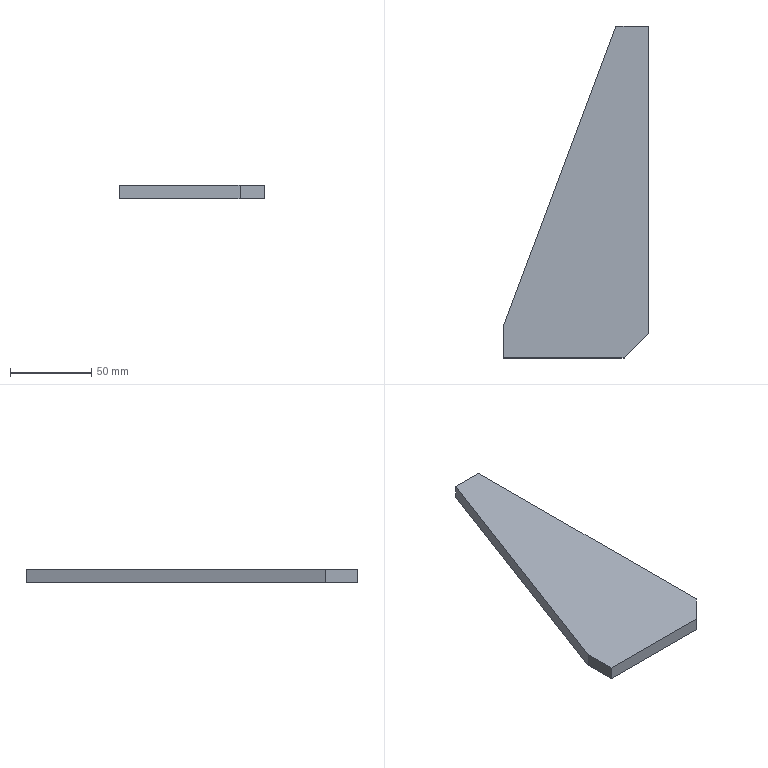Part | STEP file | 02-Rib plate | 1 solid | 8 faces | box 89 x 204 x 8 mm | volume 93564 mm3 | plane 8
STEP:
#1=CARTESIAN_POINT('',(0.,0.,0.));
#2=DIRECTION('',(0.,0.,1.));
#3=DIRECTION('',(1.,0.,0.));
#4=AXIS2_PLACEMENT_3D('',#1,#2,#3);
#5=CARTESIAN_POINT('',(0.,-189.,0.));
#6=VERTEX_POINT('',#5);
#7=CARTESIAN_POINT('',(0.,0.,0.));
#8=VERTEX_POINT('',#7);
#9=CARTESIAN_POINT('',(0.,0.,0.));
#10=DIRECTION('',(0.,1.,0.));
#11=VECTOR('',#10,1.);
#12=LINE('',#9,#11);
#13=CARTESIAN_POINT('',(0.,0.,8.));
#14=DIRECTION('',(-1.,0.,0.));
#15=DIRECTION('',(0.,-1.,0.));
#16=AXIS2_PLACEMENT_3D('',#13,#14,#15);
#17=PLANE('',#16);
#18=CARTESIAN_POINT('',(0.,-8.));
#19=DIRECTION('',(-1.,0.));
#20=VECTOR('',#19,1.);
#21=LINE('',#18,#20);
#22=(GEOMETRIC_REPRESENTATION_CONTEXT(2)PARAMETRIC_REPRESENTATION_CONTEXT()REPRESENTATION_CONTEXT('',''));
#23=DEFINITIONAL_REPRESENTATION('',(#21),#22);
#24=PCURVE('',#17,#23);
#25=CARTESIAN_POINT('',(0.,0.,0.));
#26=DIRECTION('',(0.,0.,-1.));
#27=DIRECTION('',(-1.,0.,0.));
#28=AXIS2_PLACEMENT_3D('',#25,#26,#27);
#29=PLANE('',#28);
#30=CARTESIAN_POINT('',(0.,0.));
#31=DIRECTION('',(0.,1.));
#32=VECTOR('',#31,1.);
#33=LINE('',#30,#32);
#34=(GEOMETRIC_REPRESENTATION_CONTEXT(2)PARAMETRIC_REPRESENTATION_CONTEXT()REPRESENTATION_CONTEXT('',''));
#35=DEFINITIONAL_REPRESENTATION('',(#33),#34);
#36=PCURVE('',#29,#35);
#37=SURFACE_CURVE('',#12,(#24,#36),.PCURVE_S1.);
#38=EDGE_CURVE('',#6,#8,#37,.T.);
#39=ORIENTED_EDGE('',*,*,#38,.T.);
#40=CARTESIAN_POINT('',(0.,0.,8.));
#41=VERTEX_POINT('',#40);
#42=CARTESIAN_POINT('',(0.,0.,8.));
#43=DIRECTION('',(0.,0.,-1.));
#44=VECTOR('',#43,1.);
#45=LINE('',#42,#44);
#46=CARTESIAN_POINT('',(0.,0.));
#47=DIRECTION('',(0.,-1.));
#48=VECTOR('',#47,1.);
#49=LINE('',#46,#48);
#50=(GEOMETRIC_REPRESENTATION_CONTEXT(2)PARAMETRIC_REPRESENTATION_CONTEXT()REPRESENTATION_CONTEXT('',''));
#51=DEFINITIONAL_REPRESENTATION('',(#49),#50);
#52=PCURVE('',#17,#51);
#53=CARTESIAN_POINT('',(0.,0.,8.));
#54=DIRECTION('',(0.,-1.,0.));
#55=DIRECTION('',(1.,0.,0.));
#56=AXIS2_PLACEMENT_3D('',#53,#54,#55);
#57=PLANE('',#56);
#58=CARTESIAN_POINT('',(0.,0.));
#59=DIRECTION('',(0.,-1.));
#60=VECTOR('',#59,1.);
#61=LINE('',#58,#60);
#62=(GEOMETRIC_REPRESENTATION_CONTEXT(2)PARAMETRIC_REPRESENTATION_CONTEXT()REPRESENTATION_CONTEXT('',''));
#63=DEFINITIONAL_REPRESENTATION('',(#61),#62);
#64=PCURVE('',#57,#63);
#65=SURFACE_CURVE('',#45,(#52,#64),.PCURVE_S1.);
#66=EDGE_CURVE('',#41,#8,#65,.T.);
#67=ORIENTED_EDGE('',*,*,#66,.F.);
#68=CARTESIAN_POINT('',(0.,-189.,8.));
#69=VERTEX_POINT('',#68);
#70=CARTESIAN_POINT('',(0.,0.,8.));
#71=DIRECTION('',(0.,1.,0.));
#72=VECTOR('',#71,1.);
#73=LINE('',#70,#72);
#74=CARTESIAN_POINT('',(0.,0.));
#75=DIRECTION('',(-1.,0.));
#76=VECTOR('',#75,1.);
#77=LINE('',#74,#76);
#78=(GEOMETRIC_REPRESENTATION_CONTEXT(2)PARAMETRIC_REPRESENTATION_CONTEXT()REPRESENTATION_CONTEXT('',''));
#79=DEFINITIONAL_REPRESENTATION('',(#77),#78);
#80=PCURVE('',#17,#79);
#81=CARTESIAN_POINT('',(0.,0.,8.));
#82=DIRECTION('',(0.,0.,-1.));
#83=DIRECTION('',(-1.,0.,0.));
#84=AXIS2_PLACEMENT_3D('',#81,#82,#83);
#85=PLANE('',#84);
#86=CARTESIAN_POINT('',(0.,0.));
#87=DIRECTION('',(0.,1.));
#88=VECTOR('',#87,1.);
#89=LINE('',#86,#88);
#90=(GEOMETRIC_REPRESENTATION_CONTEXT(2)PARAMETRIC_REPRESENTATION_CONTEXT()REPRESENTATION_CONTEXT('',''));
#91=DEFINITIONAL_REPRESENTATION('',(#89),#90);
#92=PCURVE('',#85,#91);
#93=SURFACE_CURVE('',#73,(#80,#92),.PCURVE_S1.);
#94=EDGE_CURVE('',#69,#41,#93,.T.);
#95=ORIENTED_EDGE('',*,*,#94,.F.);
#96=CARTESIAN_POINT('',(0.,-189.,8.));
#97=DIRECTION('',(0.,0.,-1.));
#98=VECTOR('',#97,1.);
#99=LINE('',#96,#98);
#100=CARTESIAN_POINT('',(189.,0.));
#101=DIRECTION('',(0.,-1.));
#102=VECTOR('',#101,1.);
#103=LINE('',#100,#102);
#104=(GEOMETRIC_REPRESENTATION_CONTEXT(2)PARAMETRIC_REPRESENTATION_CONTEXT()REPRESENTATION_CONTEXT('',''));
#105=DEFINITIONAL_REPRESENTATION('',(#103),#104);
#106=PCURVE('',#17,#105);
#107=CARTESIAN_POINT('',(0.,-189.,8.));
#108=DIRECTION('',(-0.7071,0.7071,0.));
#109=DIRECTION('',(-0.7071,-0.7071,0.));
#110=AXIS2_PLACEMENT_3D('',#107,#108,#109);
#111=PLANE('',#110);
#112=CARTESIAN_POINT('',(0.,0.));
#113=DIRECTION('',(0.,-1.));
#114=VECTOR('',#113,1.);
#115=LINE('',#112,#114);
#116=(GEOMETRIC_REPRESENTATION_CONTEXT(2)PARAMETRIC_REPRESENTATION_CONTEXT()REPRESENTATION_CONTEXT('',''));
#117=DEFINITIONAL_REPRESENTATION('',(#115),#116);
#118=PCURVE('',#111,#117);
#119=SURFACE_CURVE('',#99,(#106,#118),.PCURVE_S1.);
#120=EDGE_CURVE('',#69,#6,#119,.T.);
#121=ORIENTED_EDGE('',*,*,#120,.T.);
#122=EDGE_LOOP('',(#39,#67,#95,#121));
#123=FACE_BOUND('',#122,.T.);
#124=ADVANCED_FACE('',(#123),#17,.F.);
#125=CARTESIAN_POINT('',(-20.,0.,0.));
#126=VERTEX_POINT('',#125);
#127=CARTESIAN_POINT('',(0.,0.,0.));
#128=DIRECTION('',(-1.,0.,0.));
#129=VECTOR('',#128,1.);
#130=LINE('',#127,#129);
#131=CARTESIAN_POINT('',(0.,-8.));
#132=DIRECTION('',(-1.,0.));
#133=VECTOR('',#132,1.);
#134=LINE('',#131,#133);
#135=(GEOMETRIC_REPRESENTATION_CONTEXT(2)PARAMETRIC_REPRESENTATION_CONTEXT()REPRESENTATION_CONTEXT('',''));
#136=DEFINITIONAL_REPRESENTATION('',(#134),#135);
#137=PCURVE('',#57,#136);
#138=CARTESIAN_POINT('',(0.,0.));
#139=DIRECTION('',(1.,0.));
#140=VECTOR('',#139,1.);
#141=LINE('',#138,#140);
#142=(GEOMETRIC_REPRESENTATION_CONTEXT(2)PARAMETRIC_REPRESENTATION_CONTEXT()REPRESENTATION_CONTEXT('',''));
#143=DEFINITIONAL_REPRESENTATION('',(#141),#142);
#144=PCURVE('',#29,#143);
#145=SURFACE_CURVE('',#130,(#137,#144),.PCURVE_S1.);
#146=EDGE_CURVE('',#8,#126,#145,.T.);
#147=ORIENTED_EDGE('',*,*,#146,.T.);
#148=CARTESIAN_POINT('',(-20.,0.,8.));
#149=VERTEX_POINT('',#148);
#150=CARTESIAN_POINT('',(-20.,0.,8.));
#151=DIRECTION('',(0.,0.,-1.));
#152=VECTOR('',#151,1.);
#153=LINE('',#150,#152);
#154=CARTESIAN_POINT('',(-20.,0.));
#155=DIRECTION('',(0.,-1.));
#156=VECTOR('',#155,1.);
#157=LINE('',#154,#156);
#158=(GEOMETRIC_REPRESENTATION_CONTEXT(2)PARAMETRIC_REPRESENTATION_CONTEXT()REPRESENTATION_CONTEXT('',''));
#159=DEFINITIONAL_REPRESENTATION('',(#157),#158);
#160=PCURVE('',#57,#159);
#161=CARTESIAN_POINT('',(-20.,0.,8.));
#162=DIRECTION('',(0.9363,-0.3511,0.));
#163=DIRECTION('',(0.3511,0.9363,0.));
#164=AXIS2_PLACEMENT_3D('',#161,#162,#163);
#165=PLANE('',#164);
#166=CARTESIAN_POINT('',(0.,0.));
#167=DIRECTION('',(0.,-1.));
#168=VECTOR('',#167,1.);
#169=LINE('',#166,#168);
#170=(GEOMETRIC_REPRESENTATION_CONTEXT(2)PARAMETRIC_REPRESENTATION_CONTEXT()REPRESENTATION_CONTEXT('',''));
#171=DEFINITIONAL_REPRESENTATION('',(#169),#170);
#172=PCURVE('',#165,#171);
#173=SURFACE_CURVE('',#153,(#160,#172),.PCURVE_S1.);
#174=EDGE_CURVE('',#149,#126,#173,.T.);
#175=ORIENTED_EDGE('',*,*,#174,.F.);
#176=CARTESIAN_POINT('',(0.,0.,8.));
#177=DIRECTION('',(-1.,0.,0.));
#178=VECTOR('',#177,1.);
#179=LINE('',#176,#178);
#180=CARTESIAN_POINT('',(0.,0.));
#181=DIRECTION('',(-1.,0.));
#182=VECTOR('',#181,1.);
#183=LINE('',#180,#182);
#184=(GEOMETRIC_REPRESENTATION_CONTEXT(2)PARAMETRIC_REPRESENTATION_CONTEXT()REPRESENTATION_CONTEXT('',''));
#185=DEFINITIONAL_REPRESENTATION('',(#183),#184);
#186=PCURVE('',#57,#185);
#187=CARTESIAN_POINT('',(0.,0.));
#188=DIRECTION('',(1.,0.));
#189=VECTOR('',#188,1.);
#190=LINE('',#187,#189);
#191=(GEOMETRIC_REPRESENTATION_CONTEXT(2)PARAMETRIC_REPRESENTATION_CONTEXT()REPRESENTATION_CONTEXT('',''));
#192=DEFINITIONAL_REPRESENTATION('',(#190),#191);
#193=PCURVE('',#85,#192);
#194=SURFACE_CURVE('',#179,(#186,#193),.PCURVE_S1.);
#195=EDGE_CURVE('',#41,#149,#194,.T.);
#196=ORIENTED_EDGE('',*,*,#195,.F.);
#197=ORIENTED_EDGE('',*,*,#66,.T.);
#198=EDGE_LOOP('',(#147,#175,#196,#197));
#199=FACE_BOUND('',#198,.T.);
#200=ADVANCED_FACE('',(#199),#57,.F.);
#201=CARTESIAN_POINT('',(-89.,-184.,0.));
#202=VERTEX_POINT('',#201);
#203=CARTESIAN_POINT('',(-20.,0.,0.));
#204=DIRECTION('',(-0.3511,-0.9363,0.));
#205=VECTOR('',#204,1.);
#206=LINE('',#203,#205);
#207=CARTESIAN_POINT('',(0.,-8.));
#208=DIRECTION('',(-1.,0.));
#209=VECTOR('',#208,1.);
#210=LINE('',#207,#209);
#211=(GEOMETRIC_REPRESENTATION_CONTEXT(2)PARAMETRIC_REPRESENTATION_CONTEXT()REPRESENTATION_CONTEXT('',''));
#212=DEFINITIONAL_REPRESENTATION('',(#210),#211);
#213=PCURVE('',#165,#212);
#214=CARTESIAN_POINT('',(20.,0.));
#215=DIRECTION('',(0.3511,-0.9363));
#216=VECTOR('',#215,1.);
#217=LINE('',#214,#216);
#218=(GEOMETRIC_REPRESENTATION_CONTEXT(2)PARAMETRIC_REPRESENTATION_CONTEXT()REPRESENTATION_CONTEXT('',''));
#219=DEFINITIONAL_REPRESENTATION('',(#217),#218);
#220=PCURVE('',#29,#219);
#221=SURFACE_CURVE('',#206,(#213,#220),.PCURVE_S1.);
#222=EDGE_CURVE('',#126,#202,#221,.T.);
#223=ORIENTED_EDGE('',*,*,#222,.T.);
#224=CARTESIAN_POINT('',(-89.,-184.,8.));
#225=VERTEX_POINT('',#224);
#226=CARTESIAN_POINT('',(-89.,-184.,8.));
#227=DIRECTION('',(0.,0.,-1.));
#228=VECTOR('',#227,1.);
#229=LINE('',#226,#228);
#230=CARTESIAN_POINT('',(-196.512,0.));
#231=DIRECTION('',(0.,-1.));
#232=VECTOR('',#231,1.);
#233=LINE('',#230,#232);
#234=(GEOMETRIC_REPRESENTATION_CONTEXT(2)PARAMETRIC_REPRESENTATION_CONTEXT()REPRESENTATION_CONTEXT('',''));
#235=DEFINITIONAL_REPRESENTATION('',(#233),#234);
#236=PCURVE('',#165,#235);
#237=CARTESIAN_POINT('',(-89.,-184.,8.));
#238=DIRECTION('',(1.,0.,0.));
#239=DIRECTION('',(0.,0.,-1.));
#240=AXIS2_PLACEMENT_3D('',#237,#238,#239);
#241=PLANE('',#240);
#242=CARTESIAN_POINT('',(0.,0.));
#243=DIRECTION('',(1.,0.));
#244=VECTOR('',#243,1.);
#245=LINE('',#242,#244);
#246=(GEOMETRIC_REPRESENTATION_CONTEXT(2)PARAMETRIC_REPRESENTATION_CONTEXT()REPRESENTATION_CONTEXT('',''));
#247=DEFINITIONAL_REPRESENTATION('',(#245),#246);
#248=PCURVE('',#241,#247);
#249=SURFACE_CURVE('',#229,(#236,#248),.PCURVE_S1.);
#250=EDGE_CURVE('',#225,#202,#249,.T.);
#251=ORIENTED_EDGE('',*,*,#250,.F.);
#252=CARTESIAN_POINT('',(-20.,0.,8.));
#253=DIRECTION('',(-0.3511,-0.9363,0.));
#254=VECTOR('',#253,1.);
#255=LINE('',#252,#254);
#256=CARTESIAN_POINT('',(0.,0.));
#257=DIRECTION('',(-1.,0.));
#258=VECTOR('',#257,1.);
#259=LINE('',#256,#258);
#260=(GEOMETRIC_REPRESENTATION_CONTEXT(2)PARAMETRIC_REPRESENTATION_CONTEXT()REPRESENTATION_CONTEXT('',''));
#261=DEFINITIONAL_REPRESENTATION('',(#259),#260);
#262=PCURVE('',#165,#261);
#263=CARTESIAN_POINT('',(20.,0.));
#264=DIRECTION('',(0.3511,-0.9363));
#265=VECTOR('',#264,1.);
#266=LINE('',#263,#265);
#267=(GEOMETRIC_REPRESENTATION_CONTEXT(2)PARAMETRIC_REPRESENTATION_CONTEXT()REPRESENTATION_CONTEXT('',''));
#268=DEFINITIONAL_REPRESENTATION('',(#266),#267);
#269=PCURVE('',#85,#268);
#270=SURFACE_CURVE('',#255,(#262,#269),.PCURVE_S1.);
#271=EDGE_CURVE('',#149,#225,#270,.T.);
#272=ORIENTED_EDGE('',*,*,#271,.F.);
#273=ORIENTED_EDGE('',*,*,#174,.T.);
#274=EDGE_LOOP('',(#223,#251,#272,#273));
#275=FACE_BOUND('',#274,.T.);
#276=ADVANCED_FACE('',(#275),#165,.F.);
#277=CARTESIAN_POINT('',(-89.,-204.,0.));
#278=VERTEX_POINT('',#277);
#279=CARTESIAN_POINT('',(-89.,-184.,0.));
#280=DIRECTION('',(0.,-1.,0.));
#281=VECTOR('',#280,1.);
#282=LINE('',#279,#281);
#283=CARTESIAN_POINT('',(8.,0.));
#284=DIRECTION('',(0.,-1.));
#285=VECTOR('',#284,1.);
#286=LINE('',#283,#285);
#287=(GEOMETRIC_REPRESENTATION_CONTEXT(2)PARAMETRIC_REPRESENTATION_CONTEXT()REPRESENTATION_CONTEXT('',''));
#288=DEFINITIONAL_REPRESENTATION('',(#286),#287);
#289=PCURVE('',#241,#288);
#290=CARTESIAN_POINT('',(89.,-184.));
#291=DIRECTION('',(0.,-1.));
#292=VECTOR('',#291,1.);
#293=LINE('',#290,#292);
#294=(GEOMETRIC_REPRESENTATION_CONTEXT(2)PARAMETRIC_REPRESENTATION_CONTEXT()REPRESENTATION_CONTEXT('',''));
#295=DEFINITIONAL_REPRESENTATION('',(#293),#294);
#296=PCURVE('',#29,#295);
#297=SURFACE_CURVE('',#282,(#289,#296),.PCURVE_S1.);
#298=EDGE_CURVE('',#202,#278,#297,.T.);
#299=ORIENTED_EDGE('',*,*,#298,.T.);
#300=CARTESIAN_POINT('',(-89.,-204.,8.));
#301=VERTEX_POINT('',#300);
#302=CARTESIAN_POINT('',(-89.,-204.,8.));
#303=DIRECTION('',(0.,0.,-1.));
#304=VECTOR('',#303,1.);
#305=LINE('',#302,#304);
#306=CARTESIAN_POINT('',(0.,-20.));
#307=DIRECTION('',(1.,0.));
#308=VECTOR('',#307,1.);
#309=LINE('',#306,#308);
#310=(GEOMETRIC_REPRESENTATION_CONTEXT(2)PARAMETRIC_REPRESENTATION_CONTEXT()REPRESENTATION_CONTEXT('',''));
#311=DEFINITIONAL_REPRESENTATION('',(#309),#310);
#312=PCURVE('',#241,#311);
#313=CARTESIAN_POINT('',(-15.,-204.,8.));
#314=DIRECTION('',(0.,1.,0.));
#315=DIRECTION('',(0.,0.,1.));
#316=AXIS2_PLACEMENT_3D('',#313,#314,#315);
#317=PLANE('',#316);
#318=CARTESIAN_POINT('',(0.,-74.));
#319=DIRECTION('',(-1.,0.));
#320=VECTOR('',#319,1.);
#321=LINE('',#318,#320);
#322=(GEOMETRIC_REPRESENTATION_CONTEXT(2)PARAMETRIC_REPRESENTATION_CONTEXT()REPRESENTATION_CONTEXT('',''));
#323=DEFINITIONAL_REPRESENTATION('',(#321),#322);
#324=PCURVE('',#317,#323);
#325=SURFACE_CURVE('',#305,(#312,#324),.PCURVE_S1.);
#326=EDGE_CURVE('',#301,#278,#325,.T.);
#327=ORIENTED_EDGE('',*,*,#326,.F.);
#328=CARTESIAN_POINT('',(-89.,-184.,8.));
#329=DIRECTION('',(0.,-1.,0.));
#330=VECTOR('',#329,1.);
#331=LINE('',#328,#330);
#332=CARTESIAN_POINT('',(0.,0.));
#333=DIRECTION('',(0.,-1.));
#334=VECTOR('',#333,1.);
#335=LINE('',#332,#334);
#336=(GEOMETRIC_REPRESENTATION_CONTEXT(2)PARAMETRIC_REPRESENTATION_CONTEXT()REPRESENTATION_CONTEXT('',''));
#337=DEFINITIONAL_REPRESENTATION('',(#335),#336);
#338=PCURVE('',#241,#337);
#339=CARTESIAN_POINT('',(89.,-184.));
#340=DIRECTION('',(0.,-1.));
#341=VECTOR('',#340,1.);
#342=LINE('',#339,#341);
#343=(GEOMETRIC_REPRESENTATION_CONTEXT(2)PARAMETRIC_REPRESENTATION_CONTEXT()REPRESENTATION_CONTEXT('',''));
#344=DEFINITIONAL_REPRESENTATION('',(#342),#343);
#345=PCURVE('',#85,#344);
#346=SURFACE_CURVE('',#331,(#338,#345),.PCURVE_S1.);
#347=EDGE_CURVE('',#225,#301,#346,.T.);
#348=ORIENTED_EDGE('',*,*,#347,.F.);
#349=ORIENTED_EDGE('',*,*,#250,.T.);
#350=EDGE_LOOP('',(#299,#327,#348,#349));
#351=FACE_BOUND('',#350,.T.);
#352=ADVANCED_FACE('',(#351),#241,.F.);
#353=CARTESIAN_POINT('',(-15.,-204.,0.));
#354=VERTEX_POINT('',#353);
#355=CARTESIAN_POINT('',(-15.,-204.,0.));
#356=DIRECTION('',(1.,0.,0.));
#357=VECTOR('',#356,1.);
#358=LINE('',#355,#357);
#359=CARTESIAN_POINT('',(-8.,0.));
#360=DIRECTION('',(0.,1.));
#361=VECTOR('',#360,1.);
#362=LINE('',#359,#361);
#363=(GEOMETRIC_REPRESENTATION_CONTEXT(2)PARAMETRIC_REPRESENTATION_CONTEXT()REPRESENTATION_CONTEXT('',''));
#364=DEFINITIONAL_REPRESENTATION('',(#362),#363);
#365=PCURVE('',#317,#364);
#366=CARTESIAN_POINT('',(15.,-204.));
#367=DIRECTION('',(-1.,0.));
#368=VECTOR('',#367,1.);
#369=LINE('',#366,#368);
#370=(GEOMETRIC_REPRESENTATION_CONTEXT(2)PARAMETRIC_REPRESENTATION_CONTEXT()REPRESENTATION_CONTEXT('',''));
#371=DEFINITIONAL_REPRESENTATION('',(#369),#370);
#372=PCURVE('',#29,#371);
#373=SURFACE_CURVE('',#358,(#365,#372),.PCURVE_S1.);
#374=EDGE_CURVE('',#278,#354,#373,.T.);
#375=ORIENTED_EDGE('',*,*,#374,.T.);
#376=CARTESIAN_POINT('',(-15.,-204.,8.));
#377=VERTEX_POINT('',#376);
#378=CARTESIAN_POINT('',(-15.,-204.,8.));
#379=DIRECTION('',(0.,0.,-1.));
#380=VECTOR('',#379,1.);
#381=LINE('',#378,#380);
#382=CARTESIAN_POINT('',(0.,0.));
#383=DIRECTION('',(-1.,0.));
#384=VECTOR('',#383,1.);
#385=LINE('',#382,#384);
#386=(GEOMETRIC_REPRESENTATION_CONTEXT(2)PARAMETRIC_REPRESENTATION_CONTEXT()REPRESENTATION_CONTEXT('',''));
#387=DEFINITIONAL_REPRESENTATION('',(#385),#386);
#388=PCURVE('',#317,#387);
#389=CARTESIAN_POINT('',(21.213,0.));
#390=DIRECTION('',(0.,-1.));
#391=VECTOR('',#390,1.);
#392=LINE('',#389,#391);
#393=(GEOMETRIC_REPRESENTATION_CONTEXT(2)PARAMETRIC_REPRESENTATION_CONTEXT()REPRESENTATION_CONTEXT('',''));
#394=DEFINITIONAL_REPRESENTATION('',(#392),#393);
#395=PCURVE('',#111,#394);
#396=SURFACE_CURVE('',#381,(#388,#395),.PCURVE_S1.);
#397=EDGE_CURVE('',#377,#354,#396,.T.);
#398=ORIENTED_EDGE('',*,*,#397,.F.);
#399=CARTESIAN_POINT('',(-15.,-204.,8.));
#400=DIRECTION('',(1.,0.,0.));
#401=VECTOR('',#400,1.);
#402=LINE('',#399,#401);
#403=CARTESIAN_POINT('',(0.,0.));
#404=DIRECTION('',(0.,1.));
#405=VECTOR('',#404,1.);
#406=LINE('',#403,#405);
#407=(GEOMETRIC_REPRESENTATION_CONTEXT(2)PARAMETRIC_REPRESENTATION_CONTEXT()REPRESENTATION_CONTEXT('',''));
#408=DEFINITIONAL_REPRESENTATION('',(#406),#407);
#409=PCURVE('',#317,#408);
#410=CARTESIAN_POINT('',(15.,-204.));
#411=DIRECTION('',(-1.,0.));
#412=VECTOR('',#411,1.);
#413=LINE('',#410,#412);
#414=(GEOMETRIC_REPRESENTATION_CONTEXT(2)PARAMETRIC_REPRESENTATION_CONTEXT()REPRESENTATION_CONTEXT('',''));
#415=DEFINITIONAL_REPRESENTATION('',(#413),#414);
#416=PCURVE('',#85,#415);
#417=SURFACE_CURVE('',#402,(#409,#416),.PCURVE_S1.);
#418=EDGE_CURVE('',#301,#377,#417,.T.);
#419=ORIENTED_EDGE('',*,*,#418,.F.);
#420=ORIENTED_EDGE('',*,*,#326,.T.);
#421=EDGE_LOOP('',(#375,#398,#419,#420));
#422=FACE_BOUND('',#421,.T.);
#423=ADVANCED_FACE('',(#422),#317,.F.);
#424=CARTESIAN_POINT('',(0.,-189.,0.));
#425=DIRECTION('',(0.7071,0.7071,0.));
#426=VECTOR('',#425,1.);
#427=LINE('',#424,#426);
#428=CARTESIAN_POINT('',(0.,-8.));
#429=DIRECTION('',(-1.,0.));
#430=VECTOR('',#429,1.);
#431=LINE('',#428,#430);
#432=(GEOMETRIC_REPRESENTATION_CONTEXT(2)PARAMETRIC_REPRESENTATION_CONTEXT()REPRESENTATION_CONTEXT('',''));
#433=DEFINITIONAL_REPRESENTATION('',(#431),#432);
#434=PCURVE('',#111,#433);
#435=CARTESIAN_POINT('',(0.,-189.));
#436=DIRECTION('',(-0.7071,0.7071));
#437=VECTOR('',#436,1.);
#438=LINE('',#435,#437);
#439=(GEOMETRIC_REPRESENTATION_CONTEXT(2)PARAMETRIC_REPRESENTATION_CONTEXT()REPRESENTATION_CONTEXT('',''));
#440=DEFINITIONAL_REPRESENTATION('',(#438),#439);
#441=PCURVE('',#29,#440);
#442=SURFACE_CURVE('',#427,(#434,#441),.PCURVE_S1.);
#443=EDGE_CURVE('',#354,#6,#442,.T.);
#444=ORIENTED_EDGE('',*,*,#443,.T.);
#445=ORIENTED_EDGE('',*,*,#120,.F.);
#446=CARTESIAN_POINT('',(0.,-189.,8.));
#447=DIRECTION('',(0.7071,0.7071,0.));
#448=VECTOR('',#447,1.);
#449=LINE('',#446,#448);
#450=CARTESIAN_POINT('',(0.,0.));
#451=DIRECTION('',(-1.,0.));
#452=VECTOR('',#451,1.);
#453=LINE('',#450,#452);
#454=(GEOMETRIC_REPRESENTATION_CONTEXT(2)PARAMETRIC_REPRESENTATION_CONTEXT()REPRESENTATION_CONTEXT('',''));
#455=DEFINITIONAL_REPRESENTATION('',(#453),#454);
#456=PCURVE('',#111,#455);
#457=CARTESIAN_POINT('',(0.,-189.));
#458=DIRECTION('',(-0.7071,0.7071));
#459=VECTOR('',#458,1.);
#460=LINE('',#457,#459);
#461=(GEOMETRIC_REPRESENTATION_CONTEXT(2)PARAMETRIC_REPRESENTATION_CONTEXT()REPRESENTATION_CONTEXT('',''));
#462=DEFINITIONAL_REPRESENTATION('',(#460),#461);
#463=PCURVE('',#85,#462);
#464=SURFACE_CURVE('',#449,(#456,#463),.PCURVE_S1.);
#465=EDGE_CURVE('',#377,#69,#464,.T.);
#466=ORIENTED_EDGE('',*,*,#465,.F.);
#467=ORIENTED_EDGE('',*,*,#397,.T.);
#468=EDGE_LOOP('',(#444,#445,#466,#467));
#469=FACE_BOUND('',#468,.T.);
#470=ADVANCED_FACE('',(#469),#111,.F.);
#471=ORIENTED_EDGE('',*,*,#94,.T.);
#472=ORIENTED_EDGE('',*,*,#195,.T.);
#473=ORIENTED_EDGE('',*,*,#271,.T.);
#474=ORIENTED_EDGE('',*,*,#347,.T.);
#475=ORIENTED_EDGE('',*,*,#418,.T.);
#476=ORIENTED_EDGE('',*,*,#465,.T.);
#477=EDGE_LOOP('',(#471,#472,#473,#474,#475,#476));
#478=FACE_BOUND('',#477,.T.);
#479=ADVANCED_FACE('',(#478),#85,.F.);
#480=ORIENTED_EDGE('',*,*,#38,.F.);
#481=ORIENTED_EDGE('',*,*,#443,.F.);
#482=ORIENTED_EDGE('',*,*,#374,.F.);
#483=ORIENTED_EDGE('',*,*,#298,.F.);
#484=ORIENTED_EDGE('',*,*,#222,.F.);
#485=ORIENTED_EDGE('',*,*,#146,.F.);
#486=EDGE_LOOP('',(#480,#481,#482,#483,#484,#485));
#487=FACE_BOUND('',#486,.T.);
#488=ADVANCED_FACE('',(#487),#29,.T.);
#489=CLOSED_SHELL('',(#124,#200,#276,#352,#423,#470,#479,#488));
#490=MANIFOLD_SOLID_BREP('',#489);
#491=(LENGTH_UNIT()NAMED_UNIT(*)SI_UNIT(.MILLI.,.METRE.));
#492=UNCERTAINTY_MEASURE_WITH_UNIT(LENGTH_MEASURE(0.0000001),#491,'','');
#493=(NAMED_UNIT(*)PLANE_ANGLE_UNIT()SI_UNIT($,.RADIAN.));
#494=(NAMED_UNIT(*)SI_UNIT($,.STERADIAN.)SOLID_ANGLE_UNIT());
#495=(GEOMETRIC_REPRESENTATION_CONTEXT(3)GLOBAL_UNCERTAINTY_ASSIGNED_CONTEXT((#492))GLOBAL_UNIT_ASSIGNED_CONTEXT((#491,#493,#494))REPRESENTATION_CONTEXT('',''));
#496=ADVANCED_BREP_SHAPE_REPRESENTATION('',(#4,#490),#495);